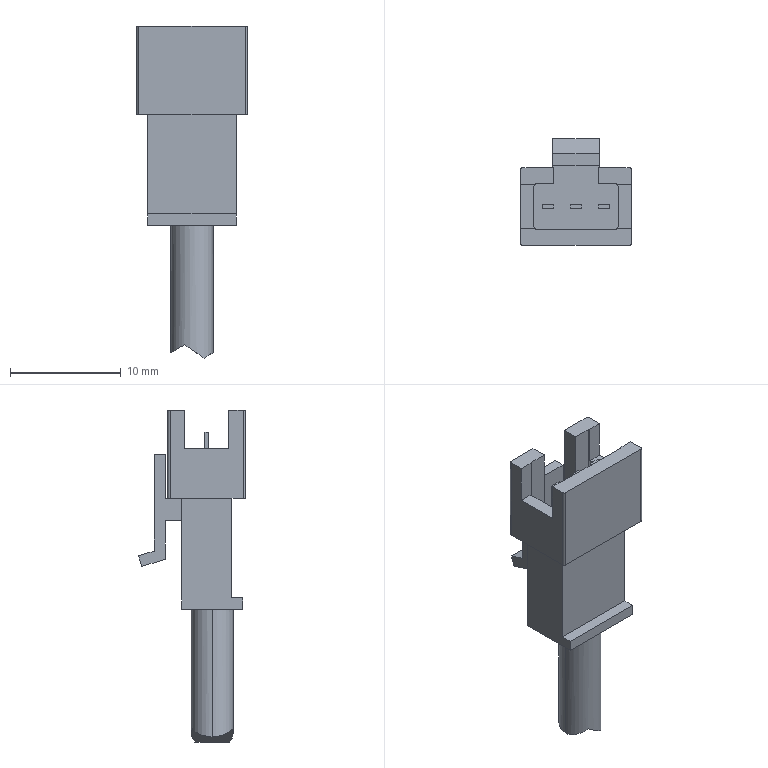Part | SolidWorks | features BaseBody 1 | 1 solid | 68 faces | box 10 x 9.65 x 30.024 mm | volume 791.952 mm3 | plane 58 | cylinder 10 | commonest cylinder face diameters 0.4 x8 3.8 x2